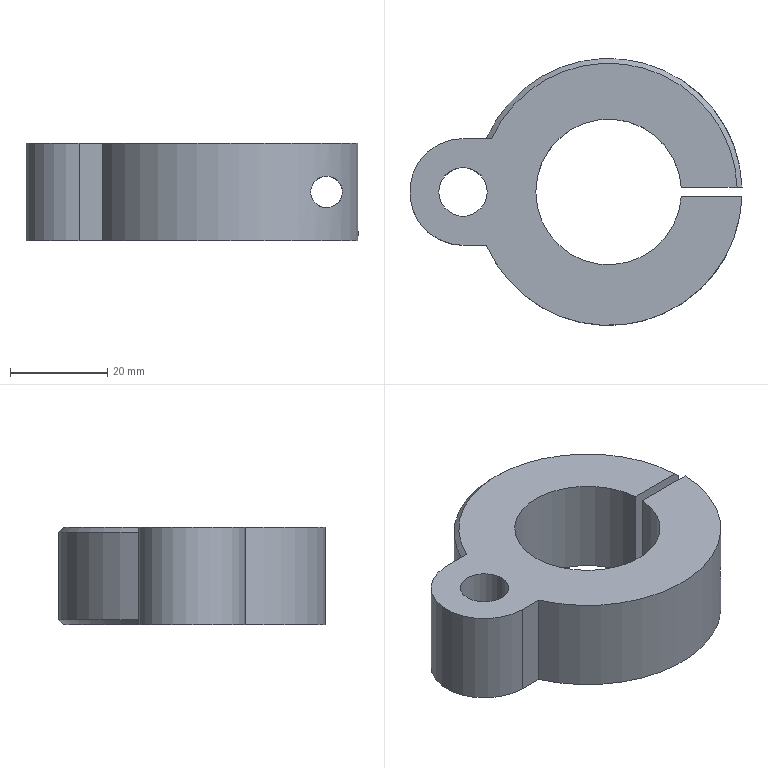Part | SolidWorks | features HoleWzd 3, Chamfer 1, Extrusion 1, ICE 1, RevCut 1 | 1 solid | 23 faces | box 68.482 x 55 x 20 mm | volume 34812 mm3 | cylinder 14 | plane 7 | cone 2 | commonest cylinder face diameters 6.5 x4 11 x3 10 x2 30 x2 55 x2 22 x1
STEP:
#1=CARTESIAN_POINT('',(21.,-17.755,3.25));
#2=VERTEX_POINT('',#1);
#3=CARTESIAN_POINT('',(21.,-17.755,-3.25));
#4=VERTEX_POINT('',#3);
#5=CARTESIAN_POINT('',(21.,-17.755,3.25));
#6=CARTESIAN_POINT('',(20.663,-18.154,3.25));
#7=CARTESIAN_POINT('',(20.32,-18.537,3.199));
#8=CARTESIAN_POINT('',(19.628,-19.268,2.969));
#9=CARTESIAN_POINT('',(19.275,-19.62,2.786));
#10=CARTESIAN_POINT('',(18.788,-20.083,2.39));
#11=CARTESIAN_POINT('',(18.63,-20.229,2.236));
#12=CARTESIAN_POINT('',(18.344,-20.489,1.887));
#13=CARTESIAN_POINT('',(18.215,-20.603,1.693));
#14=CARTESIAN_POINT('',(17.993,-20.798,1.256));
#15=CARTESIAN_POINT('',(17.905,-20.873,1.023));
#16=CARTESIAN_POINT('',(17.813,-20.951,0.6493));
#17=CARTESIAN_POINT('',(17.789,-20.971,0.5204));
#18=CARTESIAN_POINT('',(17.758,-20.998,0.2633));
#19=CARTESIAN_POINT('',(17.75,-21.004,0.134));
#20=CARTESIAN_POINT('',(17.75,-21.005,-0.1263));
#21=CARTESIAN_POINT('',(17.758,-20.998,-0.2585));
#22=CARTESIAN_POINT('',(17.789,-20.972,-0.5173));
#23=CARTESIAN_POINT('',(17.812,-20.952,-0.644));
#24=CARTESIAN_POINT('',(17.902,-20.875,-1.016));
#25=CARTESIAN_POINT('',(17.992,-20.798,-1.255));
#26=CARTESIAN_POINT('',(18.212,-20.606,-1.687));
#27=CARTESIAN_POINT('',(18.344,-20.489,-1.886));
#28=CARTESIAN_POINT('',(18.63,-20.229,-2.235));
#29=CARTESIAN_POINT('',(18.784,-20.086,-2.387));
#30=CARTESIAN_POINT('',(19.111,-19.775,-2.653));
#31=CARTESIAN_POINT('',(19.281,-19.61,-2.765));
#32=CARTESIAN_POINT('',(19.622,-19.268,-2.95));
#33=CARTESIAN_POINT('',(19.796,-19.09,-3.024));
#34=CARTESIAN_POINT('',(20.145,-18.721,-3.141));
#35=CARTESIAN_POINT('',(20.321,-18.531,-3.183));
#36=CARTESIAN_POINT('',(20.664,-18.147,-3.237));
#37=CARTESIAN_POINT('',(20.833,-17.953,-3.25));
#38=CARTESIAN_POINT('',(21.,-17.755,-3.25));
#39=B_SPLINE_CURVE_WITH_KNOTS('',3,(#5,#6,#7,#8,#9,#10,#11,#12,#13,#14,#15,#16,#17,#18,#19,#20,#21,#22,#23,#24,#25,#26,#27,#28,#29,#30,#31,#32,#33,#34,#35,#36,#37,#38),.UNSPECIFIED.,.F.,.F.,(4,2,2,2,2,2,2,2,2,2,2,2,2,2,2,2,4),(0.,0.001546,0.003091,0.003864,0.004637,0.005409,0.005796,0.006182,0.006568,0.006955,0.007728,0.0085,0.009273,0.01005,0.01082,0.01159,0.01236),.UNSPECIFIED.);
#40=EDGE_CURVE('',#2,#4,#39,.T.);
#41=ORIENTED_EDGE('',*,*,#40,.T.);
#42=CARTESIAN_POINT('',(21.,-1.,-3.25));
#43=VERTEX_POINT('',#42);
#44=CARTESIAN_POINT('',(21.,22.716,-3.25));
#45=DIRECTION('',(0.,1.,0.));
#46=VECTOR('',#45,1000.);
#47=LINE('',#44,#46);
#48=EDGE_CURVE('',#4,#43,#47,.T.);
#49=ORIENTED_EDGE('',*,*,#48,.T.);
#50=CARTESIAN_POINT('',(21.,-1.,3.25));
#51=VERTEX_POINT('',#50);
#52=CARTESIAN_POINT('',(21.,-1.,0.));
#53=DIRECTION('',(0.,-1.,0.));
#54=DIRECTION('',(1.,0.,0.));
#55=AXIS2_PLACEMENT_3D('',#52,#53,#54);
#56=CIRCLE('',#55,3.25);
#57=EDGE_CURVE('',#51,#43,#56,.T.);
#58=ORIENTED_EDGE('',*,*,#57,.F.);
#59=CARTESIAN_POINT('',(21.,22.716,3.25));
#60=DIRECTION('',(0.,1.,0.));
#61=VECTOR('',#60,1000.);
#62=LINE('',#59,#61);
#63=EDGE_CURVE('',#2,#51,#62,.T.);
#64=ORIENTED_EDGE('',*,*,#63,.F.);
#65=EDGE_LOOP('',(#41,#49,#58,#64));
#66=FACE_OUTER_BOUND('',#65,.T.);
#67=CARTESIAN_POINT('',(21.,22.716,0.));
#68=DIRECTION('',(0.,1.,0.));
#69=DIRECTION('',(0.,0.,1.));
#70=AXIS2_PLACEMENT_3D('',#67,#68,#69);
#71=CYLINDRICAL_SURFACE('',#70,3.25);
#72=ADVANCED_FACE('',(#66),#71,.F.);
#73=CARTESIAN_POINT('',(21.,8.,-5.5));
#74=VERTEX_POINT('',#73);
#75=CARTESIAN_POINT('',(21.,8.,5.5));
#76=VERTEX_POINT('',#75);
#77=CARTESIAN_POINT('',(21.,8.,0.));
#78=DIRECTION('',(0.,1.,0.));
#79=DIRECTION('',(0.,0.,1.));
#80=AXIS2_PLACEMENT_3D('',#77,#78,#79);
#81=CIRCLE('',#80,5.5);
#82=EDGE_CURVE('',#74,#76,#81,.T.);
#83=ORIENTED_EDGE('',*,*,#82,.F.);
#84=CARTESIAN_POINT('',(21.,17.755,-5.5));
#85=VERTEX_POINT('',#84);
#86=CARTESIAN_POINT('',(21.,22.716,-5.5));
#87=DIRECTION('',(0.,1.,0.));
#88=VECTOR('',#87,1000.);
#89=LINE('',#86,#88);
#90=EDGE_CURVE('',#74,#85,#89,.T.);
#91=ORIENTED_EDGE('',*,*,#90,.T.);
#92=CARTESIAN_POINT('',(21.,17.755,5.5));
#93=VERTEX_POINT('',#92);
#94=CARTESIAN_POINT('',(21.,17.755,-5.5));
#95=CARTESIAN_POINT('',(20.724,18.082,-5.5));
#96=CARTESIAN_POINT('',(20.437,18.405,-5.479));
#97=CARTESIAN_POINT('',(19.858,19.029,-5.388));
#98=CARTESIAN_POINT('',(19.565,19.33,-5.319));
#99=CARTESIAN_POINT('',(19.12,19.767,-5.171));
#100=CARTESIAN_POINT('',(18.971,19.91,-5.115));
#101=CARTESIAN_POINT('',(18.672,20.19,-4.986));
#102=CARTESIAN_POINT('',(18.522,20.328,-4.913));
#103=CARTESIAN_POINT('',(18.078,20.727,-4.671));
#104=CARTESIAN_POINT('',(17.788,20.975,-4.479));
#105=CARTESIAN_POINT('',(17.23,21.436,-4.021));
#106=CARTESIAN_POINT('',(16.96,21.649,-3.752));
#107=CARTESIAN_POINT('',(16.597,21.927,-3.302));
#108=CARTESIAN_POINT('',(16.482,22.014,-3.143));
#109=CARTESIAN_POINT('',(16.267,22.173,-2.809));
#110=CARTESIAN_POINT('',(16.166,22.247,-2.631));
#111=CARTESIAN_POINT('',(15.892,22.444,-2.08));
#112=CARTESIAN_POINT('',(15.749,22.544,-1.69));
#113=CARTESIAN_POINT('',(15.601,22.646,-1.072));
#114=CARTESIAN_POINT('',(15.563,22.672,-0.8589));
#115=CARTESIAN_POINT('',(15.513,22.707,-0.433));
#116=CARTESIAN_POINT('',(15.5,22.715,-0.2196));
#117=CARTESIAN_POINT('',(15.5,22.716,0.4218));
#118=CARTESIAN_POINT('',(15.551,22.681,0.8568));
#119=CARTESIAN_POINT('',(15.697,22.58,1.475));
#120=CARTESIAN_POINT('',(15.757,22.538,1.676));
#121=CARTESIAN_POINT('',(15.9,22.438,2.07));
#122=CARTESIAN_POINT('',(15.983,22.379,2.263));
#123=CARTESIAN_POINT('',(16.256,22.182,2.813));
#124=CARTESIAN_POINT('',(16.474,22.022,3.149));
#125=CARTESIAN_POINT('',(16.964,21.647,3.756));
#126=CARTESIAN_POINT('',(17.229,21.437,4.02));
#127=CARTESIAN_POINT('',(17.65,21.09,4.365));
#128=CARTESIAN_POINT('',(17.794,20.968,4.473));
#129=CARTESIAN_POINT('',(18.085,20.717,4.667));
#130=CARTESIAN_POINT('',(18.232,20.589,4.756));
#131=CARTESIAN_POINT('',(18.674,20.192,4.995));
#132=CARTESIAN_POINT('',(18.971,19.913,5.122));
#133=CARTESIAN_POINT('',(19.567,19.327,5.319));
#134=CARTESIAN_POINT('',(19.865,19.021,5.39));
#135=CARTESIAN_POINT('',(20.443,18.399,5.48));
#136=CARTESIAN_POINT('',(20.725,18.08,5.5));
#137=CARTESIAN_POINT('',(21.,17.755,5.5));
#138=B_SPLINE_CURVE_WITH_KNOTS('',3,(#94,#95,#96,#97,#98,#99,#100,#101,#102,#103,#104,#105,#106,#107,#108,#109,#110,#111,#112,#113,#114,#115,#116,#117,#118,#119,#120,#121,#122,#123,#124,#125,#126,#127,#128,#129,#130,#131,#132,#133,#134,#135,#136,#137),.UNSPECIFIED.,.F.,.F.,(4,2,2,2,2,2,2,2,2,2,2,2,2,2,2,2,2,2,2,2,2,4),(0.01213,0.01341,0.01469,0.01533,0.01597,0.01724,0.01852,0.01916,0.0198,0.02108,0.02172,0.02236,0.02364,0.02427,0.02491,0.02619,0.02747,0.02811,0.02875,0.03003,0.03131,0.03258),.UNSPECIFIED.);
#139=EDGE_CURVE('',#85,#93,#138,.T.);
#140=ORIENTED_EDGE('',*,*,#139,.T.);
#141=CARTESIAN_POINT('',(21.,22.716,5.5));
#142=DIRECTION('',(0.,1.,0.));
#143=VECTOR('',#142,1000.);
#144=LINE('',#141,#143);
#145=EDGE_CURVE('',#76,#93,#144,.T.);
#146=ORIENTED_EDGE('',*,*,#145,.F.);
#147=EDGE_LOOP('',(#83,#91,#140,#146));
#148=FACE_OUTER_BOUND('',#147,.T.);
#149=CARTESIAN_POINT('',(21.,22.716,0.));
#150=DIRECTION('',(0.,1.,0.));
#151=DIRECTION('',(0.,0.,1.));
#152=AXIS2_PLACEMENT_3D('',#149,#150,#151);
#153=CYLINDRICAL_SURFACE('',#152,5.5);
#154=ADVANCED_FACE('',(#148),#153,.F.);
#155=CARTESIAN_POINT('',(26.311,8.,1.431));
#156=VERTEX_POINT('',#155);
#157=CARTESIAN_POINT('',(21.,8.,0.));
#158=DIRECTION('',(0.,1.,0.));
#159=DIRECTION('',(0.,0.,1.));
#160=AXIS2_PLACEMENT_3D('',#157,#158,#159);
#161=CIRCLE('',#160,5.5);
#162=EDGE_CURVE('',#76,#156,#161,.T.);
#163=ORIENTED_EDGE('',*,*,#162,.F.);
#164=ORIENTED_EDGE('',*,*,#145,.T.);
#165=CARTESIAN_POINT('',(21.,17.755,5.5));
#166=CARTESIAN_POINT('',(21.326,17.37,5.5));
#167=CARTESIAN_POINT('',(21.642,16.975,5.471));
#168=CARTESIAN_POINT('',(22.252,16.166,5.365));
#169=CARTESIAN_POINT('',(22.542,15.759,5.288));
#170=CARTESIAN_POINT('',(23.369,14.53,4.998));
#171=CARTESIAN_POINT('',(23.865,13.698,4.728));
#172=CARTESIAN_POINT('',(24.533,12.433,4.224));
#173=CARTESIAN_POINT('',(24.744,12.008,4.039));
#174=CARTESIAN_POINT('',(25.136,11.165,3.636));
#175=CARTESIAN_POINT('',(25.317,10.746,3.42));
#176=CARTESIAN_POINT('',(25.653,9.919,2.947));
#177=CARTESIAN_POINT('',(25.807,9.509,2.692));
#178=CARTESIAN_POINT('',(26.016,8.913,2.261));
#179=CARTESIAN_POINT('',(26.082,8.719,2.11));
#180=CARTESIAN_POINT('',(26.204,8.346,1.789));
#181=CARTESIAN_POINT('',(26.26,8.166,1.619));
#182=CARTESIAN_POINT('',(26.311,8.,1.431));
#183=B_SPLINE_CURVE_WITH_KNOTS('',3,(#165,#166,#167,#168,#169,#170,#171,#172,#173,#174,#175,#176,#177,#178,#179,#180,#181,#182),.UNSPECIFIED.,.F.,.F.,(4,2,2,2,2,2,2,2,4),(0.03258,0.0341,0.03561,0.03864,0.04015,0.04167,0.04318,0.04394,0.04469),.UNSPECIFIED.);
#184=EDGE_CURVE('',#93,#156,#183,.T.);
#185=ORIENTED_EDGE('',*,*,#184,.T.);
#186=EDGE_LOOP('',(#163,#164,#185));
#187=FACE_OUTER_BOUND('',#186,.T.);
#188=CARTESIAN_POINT('',(21.,22.716,0.));
#189=DIRECTION('',(0.,1.,0.));
#190=DIRECTION('',(0.,0.,1.));
#191=AXIS2_PLACEMENT_3D('',#188,#189,#190);
#192=CYLINDRICAL_SURFACE('',#191,5.5);
#193=ADVANCED_FACE('',(#187),#192,.F.);
#194=CARTESIAN_POINT('',(21.,1.,-3.25));
#195=VERTEX_POINT('',#194);
#196=CARTESIAN_POINT('',(21.,1.,3.25));
#197=VERTEX_POINT('',#196);
#198=CARTESIAN_POINT('',(21.,1.,0.));
#199=DIRECTION('',(0.,1.,0.));
#200=DIRECTION('',(-1.,0.,0.));
#201=AXIS2_PLACEMENT_3D('',#198,#199,#200);
#202=CIRCLE('',#201,3.25);
#203=EDGE_CURVE('',#195,#197,#202,.T.);
#204=ORIENTED_EDGE('',*,*,#203,.F.);
#205=CARTESIAN_POINT('',(21.,8.,-3.25));
#206=VERTEX_POINT('',#205);
#207=CARTESIAN_POINT('',(21.,22.716,-3.25));
#208=DIRECTION('',(0.,1.,0.));
#209=VECTOR('',#208,1000.);
#210=LINE('',#207,#209);
#211=EDGE_CURVE('',#195,#206,#210,.T.);
#212=ORIENTED_EDGE('',*,*,#211,.T.);
#213=CARTESIAN_POINT('',(21.,8.,3.25));
#214=VERTEX_POINT('',#213);
#215=CARTESIAN_POINT('',(21.,8.,0.));
#216=DIRECTION('',(0.,1.,0.));
#217=DIRECTION('',(0.,0.,1.));
#218=AXIS2_PLACEMENT_3D('',#215,#216,#217);
#219=CIRCLE('',#218,3.25);
#220=EDGE_CURVE('',#206,#214,#219,.T.);
#221=ORIENTED_EDGE('',*,*,#220,.T.);
#222=CARTESIAN_POINT('',(21.,22.716,3.25));
#223=DIRECTION('',(0.,1.,0.));
#224=VECTOR('',#223,1000.);
#225=LINE('',#222,#224);
#226=EDGE_CURVE('',#197,#214,#225,.T.);
#227=ORIENTED_EDGE('',*,*,#226,.F.);
#228=EDGE_LOOP('',(#204,#212,#221,#227));
#229=FACE_OUTER_BOUND('',#228,.T.);
#230=CARTESIAN_POINT('',(21.,22.716,0.));
#231=DIRECTION('',(0.,1.,0.));
#232=DIRECTION('',(0.,0.,1.));
#233=AXIS2_PLACEMENT_3D('',#230,#231,#232);
#234=CYLINDRICAL_SURFACE('',#233,3.25);
#235=ADVANCED_FACE('',(#229),#234,.F.);
#236=CARTESIAN_POINT('',(-35.,0.,-10.));
#237=VERTEX_POINT('',#236);
#238=CARTESIAN_POINT('',(-25.,0.,-10.));
#239=VERTEX_POINT('',#238);
#240=CARTESIAN_POINT('',(-30.,0.,-10.));
#241=DIRECTION('',(0.,0.,1.));
#242=DIRECTION('',(1.,0.,0.));
#243=AXIS2_PLACEMENT_3D('',#240,#241,#242);
#244=CIRCLE('',#243,5.);
#245=EDGE_CURVE('',#237,#239,#244,.T.);
#246=ORIENTED_EDGE('',*,*,#245,.F.);
#247=CARTESIAN_POINT('',(-35.,0.,10.));
#248=VERTEX_POINT('',#247);
#249=CARTESIAN_POINT('',(-35.,0.,10.));
#250=DIRECTION('',(0.,0.,1.));
#251=VECTOR('',#250,1000.);
#252=LINE('',#249,#251);
#253=EDGE_CURVE('',#237,#248,#252,.T.);
#254=ORIENTED_EDGE('',*,*,#253,.T.);
#255=CARTESIAN_POINT('',(-25.,0.,10.));
#256=VERTEX_POINT('',#255);
#257=CARTESIAN_POINT('',(-30.,0.,10.));
#258=DIRECTION('',(0.,0.,1.));
#259=DIRECTION('',(1.,0.,0.));
#260=AXIS2_PLACEMENT_3D('',#257,#258,#259);
#261=CIRCLE('',#260,5.);
#262=EDGE_CURVE('',#248,#256,#261,.T.);
#263=ORIENTED_EDGE('',*,*,#262,.T.);
#264=CARTESIAN_POINT('',(-25.,0.,10.));
#265=DIRECTION('',(0.,0.,1.));
#266=VECTOR('',#265,1000.);
#267=LINE('',#264,#266);
#268=EDGE_CURVE('',#239,#256,#267,.T.);
#269=ORIENTED_EDGE('',*,*,#268,.F.);
#270=EDGE_LOOP('',(#246,#254,#263,#269));
#271=FACE_OUTER_BOUND('',#270,.T.);
#272=CARTESIAN_POINT('',(-30.,0.,10.));
#273=DIRECTION('',(0.,0.,1.));
#274=DIRECTION('',(1.,0.,0.));
#275=AXIS2_PLACEMENT_3D('',#272,#273,#274);
#276=CYLINDRICAL_SURFACE('',#275,5.);
#277=ADVANCED_FACE('',(#271),#276,.F.);
#278=CARTESIAN_POINT('',(-15.,0.,10.));
#279=VERTEX_POINT('',#278);
#280=CARTESIAN_POINT('',(14.967,1.,10.));
#281=VERTEX_POINT('',#280);
#282=CARTESIAN_POINT('',(0.,0.,10.));
#283=DIRECTION('',(0.,0.,-1.));
#284=DIRECTION('',(-1.,0.,0.));
#285=AXIS2_PLACEMENT_3D('',#282,#283,#284);
#286=CIRCLE('',#285,15.);
#287=EDGE_CURVE('',#279,#281,#286,.T.);
#288=ORIENTED_EDGE('',*,*,#287,.F.);
#289=CARTESIAN_POINT('',(-15.,0.,-10.));
#290=VERTEX_POINT('',#289);
#291=CARTESIAN_POINT('',(-15.,0.,10.));
#292=DIRECTION('',(0.,0.,-1.));
#293=VECTOR('',#292,1000.);
#294=LINE('',#291,#293);
#295=EDGE_CURVE('',#279,#290,#294,.T.);
#296=ORIENTED_EDGE('',*,*,#295,.T.);
#297=CARTESIAN_POINT('',(14.967,1.,-10.));
#298=VERTEX_POINT('',#297);
#299=CARTESIAN_POINT('',(0.,0.,-10.));
#300=DIRECTION('',(0.,0.,-1.));
#301=DIRECTION('',(-1.,0.,0.));
#302=AXIS2_PLACEMENT_3D('',#299,#300,#301);
#303=CIRCLE('',#302,15.);
#304=EDGE_CURVE('',#290,#298,#303,.T.);
#305=ORIENTED_EDGE('',*,*,#304,.T.);
#306=CARTESIAN_POINT('',(14.967,1.,10.));
#307=DIRECTION('',(0.,0.,-1.));
#308=VECTOR('',#307,1000.);
#309=LINE('',#306,#308);
#310=EDGE_CURVE('',#281,#298,#309,.T.);
#311=ORIENTED_EDGE('',*,*,#310,.F.);
#312=EDGE_LOOP('',(#288,#296,#305,#311));
#313=FACE_OUTER_BOUND('',#312,.T.);
#314=CARTESIAN_POINT('',(0.,0.,10.));
#315=DIRECTION('',(0.,0.,-1.));
#316=DIRECTION('',(-1.,0.,0.));
#317=AXIS2_PLACEMENT_3D('',#314,#315,#316);
#318=CYLINDRICAL_SURFACE('',#317,15.);
#319=ADVANCED_FACE('',(#313),#318,.F.);
#320=CARTESIAN_POINT('',(26.311,8.,-1.431));
#321=VERTEX_POINT('',#320);
#322=CARTESIAN_POINT('',(26.311,8.,-10.));
#323=DIRECTION('',(0.,0.,-1.));
#324=VECTOR('',#323,1000.);
#325=LINE('',#322,#324);
#326=EDGE_CURVE('',#156,#321,#325,.T.);
#327=ORIENTED_EDGE('',*,*,#326,.F.);
#328=ORIENTED_EDGE('',*,*,#184,.F.);
#329=ORIENTED_EDGE('',*,*,#139,.F.);
#330=CARTESIAN_POINT('',(26.311,8.,-1.431));
#331=CARTESIAN_POINT('',(26.26,8.168,-1.62));
#332=CARTESIAN_POINT('',(26.203,8.348,-1.791));
#333=CARTESIAN_POINT('',(26.082,8.72,-2.111));
#334=CARTESIAN_POINT('',(26.016,8.913,-2.261));
#335=CARTESIAN_POINT('',(25.809,9.504,-2.688));
#336=CARTESIAN_POINT('',(25.654,9.916,-2.946));
#337=CARTESIAN_POINT('',(25.147,11.166,-3.659));
#338=CARTESIAN_POINT('',(24.758,12.007,-4.054));
#339=CARTESIAN_POINT('',(24.094,13.265,-4.556));
#340=CARTESIAN_POINT('',(23.859,13.684,-4.707));
#341=CARTESIAN_POINT('',(23.359,14.521,-4.977));
#342=CARTESIAN_POINT('',(23.093,14.941,-5.095));
#343=CARTESIAN_POINT('',(22.259,16.18,-5.386));
#344=CARTESIAN_POINT('',(21.655,16.98,-5.5));
#345=CARTESIAN_POINT('',(21.,17.755,-5.5));
#346=B_SPLINE_CURVE_WITH_KNOTS('',3,(#330,#331,#332,#333,#334,#335,#336,#337,#338,#339,#340,#341,#342,#343,#344,#345),.UNSPECIFIED.,.F.,.F.,(4,2,2,2,2,2,2,4),(0.,0.0007582,0.001516,0.003033,0.006066,0.007582,0.009098,0.01213),.UNSPECIFIED.);
#347=EDGE_CURVE('',#321,#85,#346,.T.);
#348=ORIENTED_EDGE('',*,*,#347,.F.);
#349=EDGE_LOOP('',(#327,#328,#329,#348));
#350=FACE_BOUND('',#349,.T.);
#351=CARTESIAN_POINT('',(27.482,1.,9.));
#352=VERTEX_POINT('',#351);
#353=CARTESIAN_POINT('',(27.482,1.,-9.));
#354=VERTEX_POINT('',#353);
#355=CARTESIAN_POINT('',(27.482,1.,10.));
#356=DIRECTION('',(0.,0.,-1.));
#357=VECTOR('',#356,1000.);
#358=LINE('',#355,#357);
#359=EDGE_CURVE('',#352,#354,#358,.T.);
#360=ORIENTED_EDGE('',*,*,#359,.T.);
#361=CARTESIAN_POINT('',(-25.204,11.,-9.));
#362=VERTEX_POINT('',#361);
#363=CARTESIAN_POINT('',(0.,0.,-9.));
#364=DIRECTION('',(0.,0.,1.));
#365=DIRECTION('',(1.,0.,0.));
#366=AXIS2_PLACEMENT_3D('',#363,#364,#365);
#367=CIRCLE('',#366,27.5);
#368=EDGE_CURVE('',#354,#362,#367,.T.);
#369=ORIENTED_EDGE('',*,*,#368,.T.);
#370=CARTESIAN_POINT('',(-25.204,11.,9.));
#371=VERTEX_POINT('',#370);
#372=CARTESIAN_POINT('',(-25.204,11.,-10.));
#373=DIRECTION('',(0.,0.,1.));
#374=VECTOR('',#373,1000.);
#375=LINE('',#372,#374);
#376=EDGE_CURVE('',#362,#371,#375,.T.);
#377=ORIENTED_EDGE('',*,*,#376,.T.);
#378=CARTESIAN_POINT('',(0.,0.,9.));
#379=DIRECTION('',(0.,0.,-1.));
#380=DIRECTION('',(1.,0.,0.));
#381=AXIS2_PLACEMENT_3D('',#378,#379,#380);
#382=CIRCLE('',#381,27.5);
#383=EDGE_CURVE('',#371,#352,#382,.T.);
#384=ORIENTED_EDGE('',*,*,#383,.T.);
#385=EDGE_LOOP('',(#360,#369,#377,#384));
#386=FACE_OUTER_BOUND('',#385,.T.);
#387=CARTESIAN_POINT('',(0.,0.,-10.));
#388=DIRECTION('',(0.,0.,1.));
#389=DIRECTION('',(1.,0.,0.));
#390=AXIS2_PLACEMENT_3D('',#387,#388,#389);
#391=CYLINDRICAL_SURFACE('',#390,27.5);
#392=ADVANCED_FACE('',(#350,#386),#391,.T.);
#393=ORIENTED_EDGE('',*,*,#40,.F.);
#394=CARTESIAN_POINT('',(21.,-17.755,-3.25));
#395=CARTESIAN_POINT('',(21.384,-17.301,-3.25));
#396=CARTESIAN_POINT('',(21.758,-16.828,-3.182));
#397=CARTESIAN_POINT('',(22.277,-16.126,-2.994));
#398=CARTESIAN_POINT('',(22.445,-15.892,-2.917));
#399=CARTESIAN_POINT('',(22.768,-15.426,-2.733));
#400=CARTESIAN_POINT('',(22.924,-15.192,-2.626));
#401=CARTESIAN_POINT('',(23.222,-14.733,-2.38));
#402=CARTESIAN_POINT('',(23.363,-14.508,-2.241));
#403=CARTESIAN_POINT('',(23.627,-14.074,-1.924));
#404=CARTESIAN_POINT('',(23.751,-13.863,-1.745));
#405=CARTESIAN_POINT('',(23.915,-13.577,-1.441));
#406=CARTESIAN_POINT('',(23.966,-13.486,-1.334));
#407=CARTESIAN_POINT('',(24.06,-13.318,-1.102));
#408=CARTESIAN_POINT('',(24.102,-13.241,-0.9781));
#409=CARTESIAN_POINT('',(24.173,-13.112,-0.7169));
#410=CARTESIAN_POINT('',(24.202,-13.059,-0.5767));
#411=CARTESIAN_POINT('',(24.241,-12.986,-0.2874));
#412=CARTESIAN_POINT('',(24.251,-12.968,-0.1374));
#413=CARTESIAN_POINT('',(24.249,-12.97,0.1651));
#414=CARTESIAN_POINT('',(24.238,-12.991,0.313));
#415=CARTESIAN_POINT('',(24.197,-13.067,0.6028));
#416=CARTESIAN_POINT('',(24.167,-13.122,0.7404));
#417=CARTESIAN_POINT('',(24.095,-13.254,0.9995));
#418=CARTESIAN_POINT('',(24.052,-13.332,1.123));
#419=CARTESIAN_POINT('',(23.958,-13.501,1.352));
#420=CARTESIAN_POINT('',(23.906,-13.592,1.459));
#421=CARTESIAN_POINT('',(23.742,-13.879,1.76));
#422=CARTESIAN_POINT('',(23.617,-14.091,1.938));
#423=CARTESIAN_POINT('',(23.353,-14.524,2.251));
#424=CARTESIAN_POINT('',(23.213,-14.748,2.388));
#425=CARTESIAN_POINT('',(22.917,-15.203,2.631));
#426=CARTESIAN_POINT('',(22.761,-15.436,2.738));
#427=CARTESIAN_POINT('',(22.437,-15.904,2.921));
#428=CARTESIAN_POINT('',(22.27,-16.137,2.997));
#429=CARTESIAN_POINT('',(21.753,-16.835,3.183));
#430=CARTESIAN_POINT('',(21.388,-17.296,3.25));
#431=CARTESIAN_POINT('',(21.,-17.755,3.25));
#432=B_SPLINE_CURVE_WITH_KNOTS('',3,(#394,#395,#396,#397,#398,#399,#400,#401,#402,#403,#404,#405,#406,#407,#408,#409,#410,#411,#412,#413,#414,#415,#416,#417,#418,#419,#420,#421,#422,#423,#424,#425,#426,#427,#428,#429,#430,#431),.UNSPECIFIED.,.F.,.F.,(4,2,2,2,2,2,2,2,2,2,2,2,2,2,2,2,2,2,4),(0.01236,0.01414,0.01503,0.01592,0.01681,0.0177,0.01815,0.01859,0.01904,0.01948,0.01993,0.02037,0.02082,0.02126,0.02215,0.02304,0.02393,0.02482,0.0266),.UNSPECIFIED.);
#433=EDGE_CURVE('',#4,#2,#432,.T.);
#434=ORIENTED_EDGE('',*,*,#433,.F.);
#435=EDGE_LOOP('',(#393,#434));
#436=FACE_BOUND('',#435,.T.);
#437=CARTESIAN_POINT('',(27.482,-1.,10.));
#438=VERTEX_POINT('',#437);
#439=CARTESIAN_POINT('',(27.482,-1.,-10.));
#440=VERTEX_POINT('',#439);
#441=CARTESIAN_POINT('',(27.482,-1.,10.));
#442=DIRECTION('',(0.,0.,-1.));
#443=VECTOR('',#442,1000.);
#444=LINE('',#441,#443);
#445=EDGE_CURVE('',#438,#440,#444,.T.);
#446=ORIENTED_EDGE('',*,*,#445,.F.);
#447=CARTESIAN_POINT('',(-25.204,-11.,10.));
#448=VERTEX_POINT('',#447);
#449=CARTESIAN_POINT('',(0.,0.,10.));
#450=DIRECTION('',(0.,0.,1.));
#451=DIRECTION('',(1.,0.,0.));
#452=AXIS2_PLACEMENT_3D('',#449,#450,#451);
#453=CIRCLE('',#452,27.5);
#454=EDGE_CURVE('',#448,#438,#453,.T.);
#455=ORIENTED_EDGE('',*,*,#454,.F.);
#456=CARTESIAN_POINT('',(-25.204,-11.,-10.));
#457=VERTEX_POINT('',#456);
#458=CARTESIAN_POINT('',(-25.204,-11.,-10.));
#459=DIRECTION('',(0.,0.,1.));
#460=VECTOR('',#459,1000.);
#461=LINE('',#458,#460);
#462=EDGE_CURVE('',#457,#448,#461,.T.);
#463=ORIENTED_EDGE('',*,*,#462,.F.);
#464=CARTESIAN_POINT('',(0.,0.,-10.));
#465=DIRECTION('',(0.,0.,1.));
#466=DIRECTION('',(1.,0.,0.));
#467=AXIS2_PLACEMENT_3D('',#464,#465,#466);
#468=CIRCLE('',#467,27.5);
#469=EDGE_CURVE('',#457,#440,#468,.T.);
#470=ORIENTED_EDGE('',*,*,#469,.T.);
#471=EDGE_LOOP('',(#446,#455,#463,#470));
#472=FACE_OUTER_BOUND('',#471,.T.);
#473=CARTESIAN_POINT('',(0.,0.,-10.));
#474=DIRECTION('',(0.,0.,1.));
#475=DIRECTION('',(1.,0.,0.));
#476=AXIS2_PLACEMENT_3D('',#473,#474,#475);
#477=CYLINDRICAL_SURFACE('',#476,27.5);
#478=ADVANCED_FACE('',(#436,#472),#477,.T.);
#479=CARTESIAN_POINT('',(-30.,-11.,10.));
#480=VERTEX_POINT('',#479);
#481=CARTESIAN_POINT('',(-30.,-11.,10.));
#482=DIRECTION('',(1.,0.,0.));
#483=VECTOR('',#482,1000.);
#484=LINE('',#481,#483);
#485=EDGE_CURVE('',#480,#448,#484,.T.);
#486=ORIENTED_EDGE('',*,*,#485,.F.);
#487=CARTESIAN_POINT('',(-30.,-11.,-10.));
#488=VERTEX_POINT('',#487);
#489=CARTESIAN_POINT('',(-30.,-11.,-10.));
#490=DIRECTION('',(0.,0.,1.));
#491=VECTOR('',#490,1000.);
#492=LINE('',#489,#491);
#493=EDGE_CURVE('',#488,#480,#492,.T.);
#494=ORIENTED_EDGE('',*,*,#493,.F.);
#495=CARTESIAN_POINT('',(-30.,-11.,-10.));
#496=DIRECTION('',(1.,0.,0.));
#497=VECTOR('',#496,1000.);
#498=LINE('',#495,#497);
#499=EDGE_CURVE('',#488,#457,#498,.T.);
#500=ORIENTED_EDGE('',*,*,#499,.T.);
#501=ORIENTED_EDGE('',*,*,#462,.T.);
#502=EDGE_LOOP('',(#486,#494,#500,#501));
#503=FACE_OUTER_BOUND('',#502,.T.);
#504=CARTESIAN_POINT('',(-30.,-11.,-10.));
#505=DIRECTION('',(0.,-1.,0.));
#506=DIRECTION('',(0.,0.,-1.));
#507=AXIS2_PLACEMENT_3D('',#504,#505,#506);
#508=PLANE('',#507);
#509=ADVANCED_FACE('',(#503),#508,.T.);
#510=CARTESIAN_POINT('',(-30.,11.,10.));
#511=VERTEX_POINT('',#510);
#512=CARTESIAN_POINT('',(-30.,0.,10.));
#513=DIRECTION('',(0.,0.,1.));
#514=DIRECTION('',(1.,0.,0.));
#515=AXIS2_PLACEMENT_3D('',#512,#513,#514);
#516=CIRCLE('',#515,11.);
#517=EDGE_CURVE('',#511,#480,#516,.T.);
#518=ORIENTED_EDGE('',*,*,#517,.F.);
#519=CARTESIAN_POINT('',(-30.,11.,-10.));
#520=VERTEX_POINT('',#519);
#521=CARTESIAN_POINT('',(-30.,11.,-10.));
#522=DIRECTION('',(0.,0.,1.));
#523=VECTOR('',#522,1000.);
#524=LINE('',#521,#523);
#525=EDGE_CURVE('',#520,#511,#524,.T.);
#526=ORIENTED_EDGE('',*,*,#525,.F.);
#527=CARTESIAN_POINT('',(-30.,0.,-10.));
#528=DIRECTION('',(0.,0.,1.));
#529=DIRECTION('',(1.,0.,0.));
#530=AXIS2_PLACEMENT_3D('',#527,#528,#529);
#531=CIRCLE('',#530,11.);
#532=EDGE_CURVE('',#520,#488,#531,.T.);
#533=ORIENTED_EDGE('',*,*,#532,.T.);
#534=ORIENTED_EDGE('',*,*,#493,.T.);
#535=EDGE_LOOP('',(#518,#526,#533,#534));
#536=FACE_OUTER_BOUND('',#535,.T.);
#537=CARTESIAN_POINT('',(-30.,0.,-10.));
#538=DIRECTION('',(0.,0.,1.));
#539=DIRECTION('',(1.,0.,0.));
#540=AXIS2_PLACEMENT_3D('',#537,#538,#539);
#541=CYLINDRICAL_SURFACE('',#540,11.);
#542=ADVANCED_FACE('',(#536),#541,.T.);
#543=CARTESIAN_POINT('',(-24.109,11.,10.));
#544=VERTEX_POINT('',#543);
#545=CARTESIAN_POINT('',(-25.204,11.,10.));
#546=DIRECTION('',(-1.,0.,0.));
#547=VECTOR('',#546,1000.);
#548=LINE('',#545,#547);
#549=EDGE_CURVE('',#544,#511,#548,.T.);
#550=ORIENTED_EDGE('',*,*,#549,.F.);
#551=CARTESIAN_POINT('',(-24.109,11.,10.));
#552=CARTESIAN_POINT('',(-24.475,11.,9.667));
#553=CARTESIAN_POINT('',(-24.84,11.,9.334));
#554=CARTESIAN_POINT('',(-25.204,11.,9.));
#555=B_SPLINE_CURVE_WITH_KNOTS('',3,(#551,#552,#553,#554),.UNSPECIFIED.,.F.,.F.,(4,4),(0.,0.001483),.UNSPECIFIED.);
#556=EDGE_CURVE('',#544,#371,#555,.T.);
#557=ORIENTED_EDGE('',*,*,#556,.T.);
#558=ORIENTED_EDGE('',*,*,#376,.F.);
#559=CARTESIAN_POINT('',(-24.109,11.,-10.));
#560=VERTEX_POINT('',#559);
#561=CARTESIAN_POINT('',(-25.204,11.,-9.));
#562=CARTESIAN_POINT('',(-24.84,11.,-9.334));
#563=CARTESIAN_POINT('',(-24.475,11.,-9.667));
#564=CARTESIAN_POINT('',(-24.109,11.,-10.));
#565=B_SPLINE_CURVE_WITH_KNOTS('',3,(#561,#562,#563,#564),.UNSPECIFIED.,.F.,.F.,(4,4),(0.,0.001483),.UNSPECIFIED.);
#566=EDGE_CURVE('',#362,#560,#565,.T.);
#567=ORIENTED_EDGE('',*,*,#566,.T.);
#568=CARTESIAN_POINT('',(-25.204,11.,-10.));
#569=DIRECTION('',(-1.,0.,0.));
#570=VECTOR('',#569,1000.);
#571=LINE('',#568,#570);
#572=EDGE_CURVE('',#560,#520,#571,.T.);
#573=ORIENTED_EDGE('',*,*,#572,.T.);
#574=ORIENTED_EDGE('',*,*,#525,.T.);
#575=EDGE_LOOP('',(#550,#557,#558,#567,#573,#574));
#576=FACE_OUTER_BOUND('',#575,.T.);
#577=CARTESIAN_POINT('',(-25.204,11.,-10.));
#578=DIRECTION('',(0.,1.,0.));
#579=DIRECTION('',(-1.,0.,0.));
#580=AXIS2_PLACEMENT_3D('',#577,#578,#579);
#581=PLANE('',#580);
#582=ADVANCED_FACE('',(#576),#581,.T.);
#583=CARTESIAN_POINT('',(-30.,0.,-10.));
#584=DIRECTION('',(0.,0.,1.));
#585=DIRECTION('',(1.,0.,0.));
#586=AXIS2_PLACEMENT_3D('',#583,#584,#585);
#587=CIRCLE('',#586,5.);
#588=EDGE_CURVE('',#239,#237,#587,.T.);
#589=ORIENTED_EDGE('',*,*,#588,.T.);
#590=ORIENTED_EDGE('',*,*,#245,.T.);
#591=EDGE_LOOP('',(#589,#590));
#592=FACE_BOUND('',#591,.T.);
#593=ORIENTED_EDGE('',*,*,#572,.F.);
#594=CARTESIAN_POINT('',(26.481,1.,-10.));
#595=VERTEX_POINT('',#594);
#596=CARTESIAN_POINT('',(0.,0.,-10.));
#597=DIRECTION('',(0.,0.,-1.));
#598=DIRECTION('',(1.,0.,0.));
#599=AXIS2_PLACEMENT_3D('',#596,#597,#598);
#600=CIRCLE('',#599,26.5);
#601=EDGE_CURVE('',#560,#595,#600,.T.);
#602=ORIENTED_EDGE('',*,*,#601,.T.);
#603=CARTESIAN_POINT('',(14.967,1.,-10.));
#604=DIRECTION('',(1.,0.,0.));
#605=VECTOR('',#604,1000.);
#606=LINE('',#603,#605);
#607=EDGE_CURVE('',#298,#595,#606,.T.);
#608=ORIENTED_EDGE('',*,*,#607,.F.);
#609=ORIENTED_EDGE('',*,*,#304,.F.);
#610=CARTESIAN_POINT('',(14.967,-1.,-10.));
#611=VERTEX_POINT('',#610);
#612=CARTESIAN_POINT('',(0.,0.,-10.));
#613=DIRECTION('',(0.,0.,-1.));
#614=DIRECTION('',(-1.,0.,0.));
#615=AXIS2_PLACEMENT_3D('',#612,#613,#614);
#616=CIRCLE('',#615,15.);
#617=EDGE_CURVE('',#611,#290,#616,.T.);
#618=ORIENTED_EDGE('',*,*,#617,.F.);
#619=CARTESIAN_POINT('',(27.482,-1.,-10.));
#620=DIRECTION('',(-1.,0.,0.));
#621=VECTOR('',#620,1000.);
#622=LINE('',#619,#621);
#623=EDGE_CURVE('',#440,#611,#622,.T.);
#624=ORIENTED_EDGE('',*,*,#623,.F.);
#625=ORIENTED_EDGE('',*,*,#469,.F.);
#626=ORIENTED_EDGE('',*,*,#499,.F.);
#627=ORIENTED_EDGE('',*,*,#532,.F.);
#628=EDGE_LOOP('',(#593,#602,#608,#609,#618,#624,#625,#626,#627));
#629=FACE_OUTER_BOUND('',#628,.T.);
#630=CARTESIAN_POINT('',(0.,0.,-10.));
#631=DIRECTION('',(0.,0.,1.));
#632=DIRECTION('',(1.,0.,0.));
#633=AXIS2_PLACEMENT_3D('',#630,#631,#632);
#634=PLANE('',#633);
#635=ADVANCED_FACE('',(#592,#629),#634,.F.);
#636=CARTESIAN_POINT('',(-30.,0.,10.));
#637=DIRECTION('',(0.,0.,1.));
#638=DIRECTION('',(1.,0.,0.));
#639=AXIS2_PLACEMENT_3D('',#636,#637,#638);
#640=CIRCLE('',#639,5.);
#641=EDGE_CURVE('',#256,#248,#640,.T.);
#642=ORIENTED_EDGE('',*,*,#641,.F.);
#643=ORIENTED_EDGE('',*,*,#262,.F.);
#644=EDGE_LOOP('',(#642,#643));
#645=FACE_BOUND('',#644,.T.);
#646=CARTESIAN_POINT('',(26.481,1.,10.));
#647=VERTEX_POINT('',#646);
#648=CARTESIAN_POINT('',(14.967,1.,10.));
#649=DIRECTION('',(1.,0.,0.));
#650=VECTOR('',#649,1000.);
#651=LINE('',#648,#650);
#652=EDGE_CURVE('',#281,#647,#651,.T.);
#653=ORIENTED_EDGE('',*,*,#652,.T.);
#654=CARTESIAN_POINT('',(0.,0.,10.));
#655=DIRECTION('',(0.,0.,1.));
#656=DIRECTION('',(1.,0.,0.));
#657=AXIS2_PLACEMENT_3D('',#654,#655,#656);
#658=CIRCLE('',#657,26.5);
#659=EDGE_CURVE('',#647,#544,#658,.T.);
#660=ORIENTED_EDGE('',*,*,#659,.T.);
#661=ORIENTED_EDGE('',*,*,#549,.T.);
#662=ORIENTED_EDGE('',*,*,#517,.T.);
#663=ORIENTED_EDGE('',*,*,#485,.T.);
#664=ORIENTED_EDGE('',*,*,#454,.T.);
#665=CARTESIAN_POINT('',(14.967,-1.,10.));
#666=VERTEX_POINT('',#665);
#667=CARTESIAN_POINT('',(27.482,-1.,10.));
#668=DIRECTION('',(-1.,0.,0.));
#669=VECTOR('',#668,1000.);
#670=LINE('',#667,#669);
#671=EDGE_CURVE('',#438,#666,#670,.T.);
#672=ORIENTED_EDGE('',*,*,#671,.T.);
#673=CARTESIAN_POINT('',(0.,0.,10.));
#674=DIRECTION('',(0.,0.,-1.));
#675=DIRECTION('',(-1.,0.,0.));
#676=AXIS2_PLACEMENT_3D('',#673,#674,#675);
#677=CIRCLE('',#676,15.);
#678=EDGE_CURVE('',#666,#279,#677,.T.);
#679=ORIENTED_EDGE('',*,*,#678,.T.);
#680=ORIENTED_EDGE('',*,*,#287,.T.);
#681=EDGE_LOOP('',(#653,#660,#661,#662,#663,#664,#672,#679,#680));
#682=FACE_OUTER_BOUND('',#681,.T.);
#683=CARTESIAN_POINT('',(0.,0.,10.));
#684=DIRECTION('',(0.,0.,1.));
#685=DIRECTION('',(1.,0.,0.));
#686=AXIS2_PLACEMENT_3D('',#683,#684,#685);
#687=PLANE('',#686);
#688=ADVANCED_FACE('',(#645,#682),#687,.T.);
#689=CARTESIAN_POINT('',(21.,1.,0.));
#690=DIRECTION('',(0.,1.,0.));
#691=DIRECTION('',(-1.,0.,0.));
#692=AXIS2_PLACEMENT_3D('',#689,#690,#691);
#693=CIRCLE('',#692,3.25);
#694=EDGE_CURVE('',#197,#195,#693,.T.);
#695=ORIENTED_EDGE('',*,*,#694,.T.);
#696=ORIENTED_EDGE('',*,*,#203,.T.);
#697=EDGE_LOOP('',(#695,#696));
#698=FACE_BOUND('',#697,.T.);
#699=ORIENTED_EDGE('',*,*,#607,.T.);
#700=CARTESIAN_POINT('',(26.481,1.,-10.));
#701=CARTESIAN_POINT('',(26.815,1.,-9.667));
#702=CARTESIAN_POINT('',(27.148,1.,-9.333));
#703=CARTESIAN_POINT('',(27.482,1.,-9.));
#704=B_SPLINE_CURVE_WITH_KNOTS('',3,(#700,#701,#702,#703),.UNSPECIFIED.,.F.,.F.,(4,4),(0.,0.001415),.UNSPECIFIED.);
#705=EDGE_CURVE('',#595,#354,#704,.T.);
#706=ORIENTED_EDGE('',*,*,#705,.T.);
#707=ORIENTED_EDGE('',*,*,#359,.F.);
#708=CARTESIAN_POINT('',(27.482,1.,9.));
#709=CARTESIAN_POINT('',(27.148,1.,9.333));
#710=CARTESIAN_POINT('',(26.815,1.,9.667));
#711=CARTESIAN_POINT('',(26.481,1.,10.));
#712=B_SPLINE_CURVE_WITH_KNOTS('',3,(#708,#709,#710,#711),.UNSPECIFIED.,.F.,.F.,(4,4),(0.,0.001415),.UNSPECIFIED.);
#713=EDGE_CURVE('',#352,#647,#712,.T.);
#714=ORIENTED_EDGE('',*,*,#713,.T.);
#715=ORIENTED_EDGE('',*,*,#652,.F.);
#716=ORIENTED_EDGE('',*,*,#310,.T.);
#717=EDGE_LOOP('',(#699,#706,#707,#714,#715,#716));
#718=FACE_OUTER_BOUND('',#717,.T.);
#719=CARTESIAN_POINT('',(14.967,1.,10.));
#720=DIRECTION('',(0.,1.,0.));
#721=DIRECTION('',(-1.,0.,0.));
#722=AXIS2_PLACEMENT_3D('',#719,#720,#721);
#723=PLANE('',#722);
#724=ADVANCED_FACE('',(#698,#718),#723,.F.);
#725=ORIENTED_EDGE('',*,*,#57,.T.);
#726=CARTESIAN_POINT('',(21.,-1.,0.));
#727=DIRECTION('',(0.,-1.,0.));
#728=DIRECTION('',(1.,0.,0.));
#729=AXIS2_PLACEMENT_3D('',#726,#727,#728);
#730=CIRCLE('',#729,3.25);
#731=EDGE_CURVE('',#43,#51,#730,.T.);
#732=ORIENTED_EDGE('',*,*,#731,.T.);
#733=EDGE_LOOP('',(#725,#732));
#734=FACE_BOUND('',#733,.T.);
#735=ORIENTED_EDGE('',*,*,#623,.T.);
#736=CARTESIAN_POINT('',(14.967,-1.,10.));
#737=DIRECTION('',(0.,0.,-1.));
#738=VECTOR('',#737,1000.);
#739=LINE('',#736,#738);
#740=EDGE_CURVE('',#666,#611,#739,.T.);
#741=ORIENTED_EDGE('',*,*,#740,.F.);
#742=ORIENTED_EDGE('',*,*,#671,.F.);
#743=ORIENTED_EDGE('',*,*,#445,.T.);
#744=EDGE_LOOP('',(#735,#741,#742,#743));
#745=FACE_OUTER_BOUND('',#744,.T.);
#746=CARTESIAN_POINT('',(27.482,-1.,10.));
#747=DIRECTION('',(0.,-1.,0.));
#748=DIRECTION('',(1.,0.,0.));
#749=AXIS2_PLACEMENT_3D('',#746,#747,#748);
#750=PLANE('',#749);
#751=ADVANCED_FACE('',(#734,#745),#750,.F.);
#752=ORIENTED_EDGE('',*,*,#295,.F.);
#753=ORIENTED_EDGE('',*,*,#678,.F.);
#754=ORIENTED_EDGE('',*,*,#740,.T.);
#755=ORIENTED_EDGE('',*,*,#617,.T.);
#756=EDGE_LOOP('',(#752,#753,#754,#755));
#757=FACE_OUTER_BOUND('',#756,.T.);
#758=CARTESIAN_POINT('',(0.,0.,10.));
#759=DIRECTION('',(0.,0.,-1.));
#760=DIRECTION('',(-1.,0.,0.));
#761=AXIS2_PLACEMENT_3D('',#758,#759,#760);
#762=CYLINDRICAL_SURFACE('',#761,15.);
#763=ADVANCED_FACE('',(#757),#762,.F.);
#764=ORIENTED_EDGE('',*,*,#253,.F.);
#765=ORIENTED_EDGE('',*,*,#588,.F.);
#766=ORIENTED_EDGE('',*,*,#268,.T.);
#767=ORIENTED_EDGE('',*,*,#641,.T.);
#768=EDGE_LOOP('',(#764,#765,#766,#767));
#769=FACE_OUTER_BOUND('',#768,.T.);
#770=CARTESIAN_POINT('',(-30.,0.,10.));
#771=DIRECTION('',(0.,0.,1.));
#772=DIRECTION('',(1.,0.,0.));
#773=AXIS2_PLACEMENT_3D('',#770,#771,#772);
#774=CYLINDRICAL_SURFACE('',#773,5.);
#775=ADVANCED_FACE('',(#769),#774,.F.);
#776=ORIENTED_EDGE('',*,*,#211,.F.);
#777=ORIENTED_EDGE('',*,*,#694,.F.);
#778=ORIENTED_EDGE('',*,*,#226,.T.);
#779=CARTESIAN_POINT('',(21.,8.,0.));
#780=DIRECTION('',(0.,1.,0.));
#781=DIRECTION('',(0.,0.,1.));
#782=AXIS2_PLACEMENT_3D('',#779,#780,#781);
#783=CIRCLE('',#782,3.25);
#784=EDGE_CURVE('',#214,#206,#783,.T.);
#785=ORIENTED_EDGE('',*,*,#784,.T.);
#786=EDGE_LOOP('',(#776,#777,#778,#785));
#787=FACE_OUTER_BOUND('',#786,.T.);
#788=CARTESIAN_POINT('',(21.,22.716,0.));
#789=DIRECTION('',(0.,1.,0.));
#790=DIRECTION('',(0.,0.,1.));
#791=AXIS2_PLACEMENT_3D('',#788,#789,#790);
#792=CYLINDRICAL_SURFACE('',#791,3.25);
#793=ADVANCED_FACE('',(#787),#792,.F.);
#794=ORIENTED_EDGE('',*,*,#90,.F.);
#795=CARTESIAN_POINT('',(21.,8.,0.));
#796=DIRECTION('',(0.,1.,0.));
#797=DIRECTION('',(0.,0.,1.));
#798=AXIS2_PLACEMENT_3D('',#795,#796,#797);
#799=CIRCLE('',#798,5.5);
#800=EDGE_CURVE('',#321,#74,#799,.T.);
#801=ORIENTED_EDGE('',*,*,#800,.F.);
#802=ORIENTED_EDGE('',*,*,#347,.T.);
#803=EDGE_LOOP('',(#794,#801,#802));
#804=FACE_OUTER_BOUND('',#803,.T.);
#805=CARTESIAN_POINT('',(21.,22.716,0.));
#806=DIRECTION('',(0.,1.,0.));
#807=DIRECTION('',(0.,0.,1.));
#808=AXIS2_PLACEMENT_3D('',#805,#806,#807);
#809=CYLINDRICAL_SURFACE('',#808,5.5);
#810=ADVANCED_FACE('',(#804),#809,.F.);
#811=ORIENTED_EDGE('',*,*,#326,.T.);
#812=ORIENTED_EDGE('',*,*,#800,.T.);
#813=ORIENTED_EDGE('',*,*,#82,.T.);
#814=ORIENTED_EDGE('',*,*,#162,.T.);
#815=EDGE_LOOP('',(#811,#812,#813,#814));
#816=FACE_OUTER_BOUND('',#815,.T.);
#817=ORIENTED_EDGE('',*,*,#784,.F.);
#818=ORIENTED_EDGE('',*,*,#220,.F.);
#819=EDGE_LOOP('',(#817,#818));
#820=FACE_BOUND('',#819,.T.);
#821=CARTESIAN_POINT('',(24.25,8.,0.));
#822=DIRECTION('',(0.,-1.,0.));
#823=DIRECTION('',(0.,0.,-1.));
#824=AXIS2_PLACEMENT_3D('',#821,#822,#823);
#825=PLANE('',#824);
#826=ADVANCED_FACE('',(#816,#820),#825,.F.);
#827=ORIENTED_EDGE('',*,*,#48,.F.);
#828=ORIENTED_EDGE('',*,*,#433,.T.);
#829=ORIENTED_EDGE('',*,*,#63,.T.);
#830=ORIENTED_EDGE('',*,*,#731,.F.);
#831=EDGE_LOOP('',(#827,#828,#829,#830));
#832=FACE_OUTER_BOUND('',#831,.T.);
#833=CARTESIAN_POINT('',(21.,22.716,0.));
#834=DIRECTION('',(0.,1.,0.));
#835=DIRECTION('',(0.,0.,1.));
#836=AXIS2_PLACEMENT_3D('',#833,#834,#835);
#837=CYLINDRICAL_SURFACE('',#836,3.25);
#838=ADVANCED_FACE('',(#832),#837,.F.);
#839=ORIENTED_EDGE('',*,*,#705,.F.);
#840=ORIENTED_EDGE('',*,*,#601,.F.);
#841=ORIENTED_EDGE('',*,*,#566,.F.);
#842=ORIENTED_EDGE('',*,*,#368,.F.);
#843=EDGE_LOOP('',(#839,#840,#841,#842));
#844=FACE_OUTER_BOUND('',#843,.T.);
#845=CARTESIAN_POINT('',(0.,0.,-9.));
#846=DIRECTION('',(0.,0.,1.));
#847=DIRECTION('',(1.,0.,0.));
#848=AXIS2_PLACEMENT_3D('',#845,#846,#847);
#849=CONICAL_SURFACE('',#848,27.5,0.7854);
#850=ADVANCED_FACE('',(#844),#849,.T.);
#851=ORIENTED_EDGE('',*,*,#713,.F.);
#852=ORIENTED_EDGE('',*,*,#383,.F.);
#853=ORIENTED_EDGE('',*,*,#556,.F.);
#854=ORIENTED_EDGE('',*,*,#659,.F.);
#855=EDGE_LOOP('',(#851,#852,#853,#854));
#856=FACE_OUTER_BOUND('',#855,.T.);
#857=CARTESIAN_POINT('',(0.,0.,10.));
#858=DIRECTION('',(0.,0.,-1.));
#859=DIRECTION('',(-1.,0.,0.));
#860=AXIS2_PLACEMENT_3D('',#857,#858,#859);
#861=CONICAL_SURFACE('',#860,26.5,0.7854);
#862=ADVANCED_FACE('',(#856),#861,.T.);
#863=CLOSED_SHELL('',(#72,#154,#193,#235,#277,#319,#392,#478,#509,#542,#582,#635,#688,#724,#751,#763,#775,#793,#810,#826,#838,#850,#862));
#864=MANIFOLD_SOLID_BREP('',#863);
#865=CARTESIAN_POINT('',(0.,0.,0.));
#866=DIRECTION('',(0.,0.,1.));
#867=DIRECTION('',(1.,0.,0.));
#868=AXIS2_PLACEMENT_3D('',#865,#866,#867);
#869=(LENGTH_UNIT()NAMED_UNIT(*)SI_UNIT(.MILLI.,.METRE.));
#870=UNCERTAINTY_MEASURE_WITH_UNIT(LENGTH_MEASURE(0.00001),#869,'','');
#871=(NAMED_UNIT(*)PLANE_ANGLE_UNIT()SI_UNIT($,.RADIAN.));
#872=(NAMED_UNIT(*)SI_UNIT($,.STERADIAN.)SOLID_ANGLE_UNIT());
#873=(GEOMETRIC_REPRESENTATION_CONTEXT(3)GLOBAL_UNCERTAINTY_ASSIGNED_CONTEXT((#870))GLOBAL_UNIT_ASSIGNED_CONTEXT((#869,#871,#872))REPRESENTATION_CONTEXT('',''));
#874=ADVANCED_BREP_SHAPE_REPRESENTATION('',(#864,#868),#873);